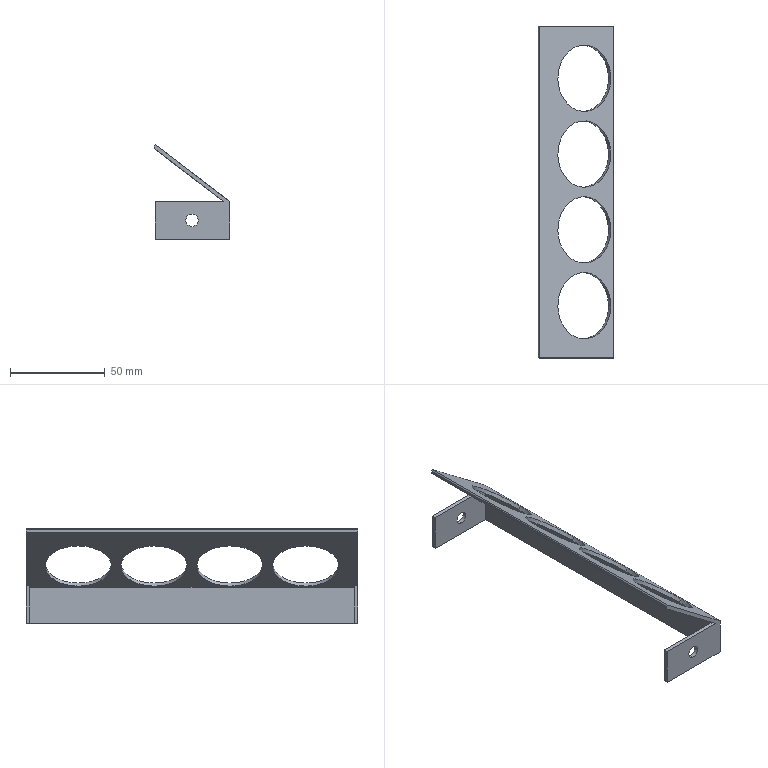Part | SolidWorks | features BaseBody 1 | 1 solid | 27 faces | box 40 x 175 x 50 mm | volume 19089 mm3 | plane 15 | cylinder 12 | commonest cylinder face diameters 35 x8 6.5 x4
STEP:
#1=CARTESIAN_POINT('',(163.696,-4210.973,1848.314));
#2=VERTEX_POINT('',#1);
#3=CARTESIAN_POINT('',(191.569,-4210.973,1827.145));
#4=VERTEX_POINT('',#3);
#5=CARTESIAN_POINT('',(163.696,-4210.973,1848.314));
#6=CARTESIAN_POINT('',(163.696,-4245.973,1848.314));
#7=CARTESIAN_POINT('',(191.569,-4245.973,1827.145));
#8=CARTESIAN_POINT('',(191.569,-4210.973,1827.145));
#9=(BOUNDED_CURVE()B_SPLINE_CURVE(3,(#5,#6,#7,#8),.UNSPECIFIED.,.F.,.F.)B_SPLINE_CURVE_WITH_KNOTS((4,4),(0.,3.142),.UNSPECIFIED.)CURVE()GEOMETRIC_REPRESENTATION_ITEM()RATIONAL_B_SPLINE_CURVE((1.,0.3333,0.3333,1.))REPRESENTATION_ITEM(''));
#10=EDGE_CURVE('',#2,#4,#9,.T.);
#11=ORIENTED_EDGE('',*,*,#10,.F.);
#12=CARTESIAN_POINT('',(164.9,-4210.973,1849.911));
#13=VERTEX_POINT('',#12);
#14=CARTESIAN_POINT('',(167.638,-4210.973,1853.544));
#15=DIRECTION('',(0.6018,0.,0.7986));
#16=VECTOR('',#15,1000.);
#17=LINE('',#14,#16);
#18=EDGE_CURVE('',#2,#13,#17,.T.);
#19=ORIENTED_EDGE('',*,*,#18,.T.);
#20=CARTESIAN_POINT('',(192.773,-4210.973,1828.742));
#21=VERTEX_POINT('',#20);
#22=CARTESIAN_POINT('',(192.773,-4210.973,1828.742));
#23=CARTESIAN_POINT('',(192.773,-4245.973,1828.742));
#24=CARTESIAN_POINT('',(164.9,-4245.973,1849.911));
#25=CARTESIAN_POINT('',(164.9,-4210.973,1849.911));
#26=(BOUNDED_CURVE()B_SPLINE_CURVE(3,(#22,#23,#24,#25),.UNSPECIFIED.,.F.,.T.)B_SPLINE_CURVE_WITH_KNOTS((4,4),(3.142,6.283),.UNSPECIFIED.)CURVE()GEOMETRIC_REPRESENTATION_ITEM()RATIONAL_B_SPLINE_CURVE((1.,0.3333,0.3333,1.))REPRESENTATION_ITEM(''));
#27=EDGE_CURVE('',#21,#13,#26,.T.);
#28=ORIENTED_EDGE('',*,*,#27,.F.);
#29=CARTESIAN_POINT('',(195.59,-4210.973,1832.481));
#30=DIRECTION('',(0.6018,0.,0.7986));
#31=VECTOR('',#30,1000.);
#32=LINE('',#29,#31);
#33=EDGE_CURVE('',#4,#21,#32,.T.);
#34=ORIENTED_EDGE('',*,*,#33,.F.);
#35=EDGE_LOOP('',(#11,#19,#28,#34));
#36=FACE_OUTER_BOUND('',#35,.T.);
#37=CARTESIAN_POINT('',(181.614,-4210.973,1843.013));
#38=DIRECTION('',(0.6018,0.,0.7986));
#39=DIRECTION('',(0.7986,0.,-0.6018));
#40=AXIS2_PLACEMENT_3D('',#37,#38,#39);
#41=CYLINDRICAL_SURFACE('',#40,17.5);
#42=ADVANCED_FACE('',(#36),#41,.F.);
#43=CARTESIAN_POINT('',(192.773,-4250.973,1828.742));
#44=VERTEX_POINT('',#43);
#45=CARTESIAN_POINT('',(164.9,-4250.973,1849.911));
#46=VERTEX_POINT('',#45);
#47=CARTESIAN_POINT('',(192.773,-4250.973,1828.742));
#48=CARTESIAN_POINT('',(192.773,-4285.973,1828.742));
#49=CARTESIAN_POINT('',(164.9,-4285.973,1849.911));
#50=CARTESIAN_POINT('',(164.9,-4250.973,1849.911));
#51=(BOUNDED_CURVE()B_SPLINE_CURVE(3,(#47,#48,#49,#50),.UNSPECIFIED.,.F.,.T.)B_SPLINE_CURVE_WITH_KNOTS((4,4),(0.,3.142),.UNSPECIFIED.)CURVE()GEOMETRIC_REPRESENTATION_ITEM()RATIONAL_B_SPLINE_CURVE((1.,0.3333,0.3333,1.))REPRESENTATION_ITEM(''));
#52=EDGE_CURVE('',#44,#46,#51,.T.);
#53=ORIENTED_EDGE('',*,*,#52,.F.);
#54=CARTESIAN_POINT('',(191.569,-4250.973,1827.145));
#55=VERTEX_POINT('',#54);
#56=CARTESIAN_POINT('',(195.59,-4250.973,1832.481));
#57=DIRECTION('',(-0.6018,0.,-0.7986));
#58=VECTOR('',#57,1000.);
#59=LINE('',#56,#58);
#60=EDGE_CURVE('',#44,#55,#59,.T.);
#61=ORIENTED_EDGE('',*,*,#60,.T.);
#62=CARTESIAN_POINT('',(163.696,-4250.973,1848.314));
#63=VERTEX_POINT('',#62);
#64=CARTESIAN_POINT('',(163.696,-4250.973,1848.314));
#65=CARTESIAN_POINT('',(163.696,-4285.973,1848.314));
#66=CARTESIAN_POINT('',(191.569,-4285.973,1827.145));
#67=CARTESIAN_POINT('',(191.569,-4250.973,1827.145));
#68=(BOUNDED_CURVE()B_SPLINE_CURVE(3,(#64,#65,#66,#67),.UNSPECIFIED.,.F.,.F.)B_SPLINE_CURVE_WITH_KNOTS((4,4),(3.142,6.283),.UNSPECIFIED.)CURVE()GEOMETRIC_REPRESENTATION_ITEM()RATIONAL_B_SPLINE_CURVE((1.,0.3333,0.3333,1.))REPRESENTATION_ITEM(''));
#69=EDGE_CURVE('',#63,#55,#68,.T.);
#70=ORIENTED_EDGE('',*,*,#69,.F.);
#71=CARTESIAN_POINT('',(167.638,-4250.973,1853.544));
#72=DIRECTION('',(-0.6018,0.,-0.7986));
#73=VECTOR('',#72,1000.);
#74=LINE('',#71,#73);
#75=EDGE_CURVE('',#46,#63,#74,.T.);
#76=ORIENTED_EDGE('',*,*,#75,.F.);
#77=EDGE_LOOP('',(#53,#61,#70,#76));
#78=FACE_OUTER_BOUND('',#77,.T.);
#79=CARTESIAN_POINT('',(181.614,-4250.973,1843.013));
#80=DIRECTION('',(-0.6018,0.,-0.7986));
#81=DIRECTION('',(-0.7986,0.,0.6018));
#82=AXIS2_PLACEMENT_3D('',#79,#80,#81);
#83=CYLINDRICAL_SURFACE('',#82,17.5);
#84=ADVANCED_FACE('',(#78),#83,.F.);
#85=CARTESIAN_POINT('',(192.773,-4290.973,1828.742));
#86=VERTEX_POINT('',#85);
#87=CARTESIAN_POINT('',(164.9,-4290.973,1849.911));
#88=VERTEX_POINT('',#87);
#89=CARTESIAN_POINT('',(192.773,-4290.973,1828.742));
#90=CARTESIAN_POINT('',(192.773,-4325.973,1828.742));
#91=CARTESIAN_POINT('',(164.9,-4325.973,1849.911));
#92=CARTESIAN_POINT('',(164.9,-4290.973,1849.911));
#93=(BOUNDED_CURVE()B_SPLINE_CURVE(3,(#89,#90,#91,#92),.UNSPECIFIED.,.F.,.T.)B_SPLINE_CURVE_WITH_KNOTS((4,4),(0.,3.142),.UNSPECIFIED.)CURVE()GEOMETRIC_REPRESENTATION_ITEM()RATIONAL_B_SPLINE_CURVE((1.,0.3333,0.3333,1.))REPRESENTATION_ITEM(''));
#94=EDGE_CURVE('',#86,#88,#93,.T.);
#95=ORIENTED_EDGE('',*,*,#94,.F.);
#96=CARTESIAN_POINT('',(191.569,-4290.973,1827.145));
#97=VERTEX_POINT('',#96);
#98=CARTESIAN_POINT('',(195.59,-4290.973,1832.481));
#99=DIRECTION('',(-0.6018,0.,-0.7986));
#100=VECTOR('',#99,1000.);
#101=LINE('',#98,#100);
#102=EDGE_CURVE('',#86,#97,#101,.T.);
#103=ORIENTED_EDGE('',*,*,#102,.T.);
#104=CARTESIAN_POINT('',(163.696,-4290.973,1848.314));
#105=VERTEX_POINT('',#104);
#106=CARTESIAN_POINT('',(163.696,-4290.973,1848.314));
#107=CARTESIAN_POINT('',(163.696,-4325.973,1848.314));
#108=CARTESIAN_POINT('',(191.569,-4325.973,1827.145));
#109=CARTESIAN_POINT('',(191.569,-4290.973,1827.145));
#110=(BOUNDED_CURVE()B_SPLINE_CURVE(3,(#106,#107,#108,#109),.UNSPECIFIED.,.F.,.F.)B_SPLINE_CURVE_WITH_KNOTS((4,4),(3.142,6.283),.UNSPECIFIED.)CURVE()GEOMETRIC_REPRESENTATION_ITEM()RATIONAL_B_SPLINE_CURVE((1.,0.3333,0.3333,1.))REPRESENTATION_ITEM(''));
#111=EDGE_CURVE('',#105,#97,#110,.T.);
#112=ORIENTED_EDGE('',*,*,#111,.F.);
#113=CARTESIAN_POINT('',(167.638,-4290.973,1853.544));
#114=DIRECTION('',(-0.6018,0.,-0.7986));
#115=VECTOR('',#114,1000.);
#116=LINE('',#113,#115);
#117=EDGE_CURVE('',#88,#105,#116,.T.);
#118=ORIENTED_EDGE('',*,*,#117,.F.);
#119=EDGE_LOOP('',(#95,#103,#112,#118));
#120=FACE_OUTER_BOUND('',#119,.T.);
#121=CARTESIAN_POINT('',(181.614,-4290.973,1843.013));
#122=DIRECTION('',(-0.6018,0.,-0.7986));
#123=DIRECTION('',(-0.7986,0.,0.6018));
#124=AXIS2_PLACEMENT_3D('',#121,#122,#123);
#125=CYLINDRICAL_SURFACE('',#124,17.5);
#126=ADVANCED_FACE('',(#120),#125,.F.);
#127=CARTESIAN_POINT('',(163.696,-4170.973,1848.314));
#128=VERTEX_POINT('',#127);
#129=CARTESIAN_POINT('',(191.569,-4170.973,1827.145));
#130=VERTEX_POINT('',#129);
#131=CARTESIAN_POINT('',(163.696,-4170.973,1848.314));
#132=CARTESIAN_POINT('',(163.696,-4205.973,1848.314));
#133=CARTESIAN_POINT('',(191.569,-4205.973,1827.145));
#134=CARTESIAN_POINT('',(191.569,-4170.973,1827.145));
#135=(BOUNDED_CURVE()B_SPLINE_CURVE(3,(#131,#132,#133,#134),.UNSPECIFIED.,.F.,.T.)B_SPLINE_CURVE_WITH_KNOTS((4,4),(0.,3.142),.UNSPECIFIED.)CURVE()GEOMETRIC_REPRESENTATION_ITEM()RATIONAL_B_SPLINE_CURVE((1.,0.3333,0.3333,1.))REPRESENTATION_ITEM(''));
#136=EDGE_CURVE('',#128,#130,#135,.T.);
#137=ORIENTED_EDGE('',*,*,#136,.F.);
#138=CARTESIAN_POINT('',(164.9,-4170.973,1849.911));
#139=VERTEX_POINT('',#138);
#140=CARTESIAN_POINT('',(167.638,-4170.973,1853.544));
#141=DIRECTION('',(0.6018,0.,0.7986));
#142=VECTOR('',#141,1000.);
#143=LINE('',#140,#142);
#144=EDGE_CURVE('',#128,#139,#143,.T.);
#145=ORIENTED_EDGE('',*,*,#144,.T.);
#146=CARTESIAN_POINT('',(192.773,-4170.973,1828.742));
#147=VERTEX_POINT('',#146);
#148=CARTESIAN_POINT('',(192.773,-4170.973,1828.742));
#149=CARTESIAN_POINT('',(192.773,-4205.973,1828.742));
#150=CARTESIAN_POINT('',(164.9,-4205.973,1849.911));
#151=CARTESIAN_POINT('',(164.9,-4170.973,1849.911));
#152=(BOUNDED_CURVE()B_SPLINE_CURVE(3,(#148,#149,#150,#151),.UNSPECIFIED.,.F.,.T.)B_SPLINE_CURVE_WITH_KNOTS((4,4),(3.142,6.283),.UNSPECIFIED.)CURVE()GEOMETRIC_REPRESENTATION_ITEM()RATIONAL_B_SPLINE_CURVE((1.,0.3333,0.3333,1.))REPRESENTATION_ITEM(''));
#153=EDGE_CURVE('',#147,#139,#152,.T.);
#154=ORIENTED_EDGE('',*,*,#153,.F.);
#155=CARTESIAN_POINT('',(195.59,-4170.973,1832.481));
#156=DIRECTION('',(0.6018,0.,0.7986));
#157=VECTOR('',#156,1000.);
#158=LINE('',#155,#157);
#159=EDGE_CURVE('',#130,#147,#158,.T.);
#160=ORIENTED_EDGE('',*,*,#159,.F.);
#161=EDGE_LOOP('',(#137,#145,#154,#160));
#162=FACE_OUTER_BOUND('',#161,.T.);
#163=CARTESIAN_POINT('',(181.614,-4170.973,1843.013));
#164=DIRECTION('',(0.6018,0.,0.7986));
#165=DIRECTION('',(0.7986,0.,-0.6018));
#166=AXIS2_PLACEMENT_3D('',#163,#164,#165);
#167=CYLINDRICAL_SURFACE('',#166,17.5);
#168=ADVANCED_FACE('',(#162),#167,.F.);
#169=CARTESIAN_POINT('',(174.446,-4143.473,1820.721));
#170=VERTEX_POINT('',#169);
#171=CARTESIAN_POINT('',(174.446,-4143.473,1814.221));
#172=VERTEX_POINT('',#171);
#173=CARTESIAN_POINT('',(174.446,-4143.473,1817.471));
#174=DIRECTION('',(0.,-1.,0.));
#175=DIRECTION('',(0.,0.,-1.));
#176=AXIS2_PLACEMENT_3D('',#173,#174,#175);
#177=CIRCLE('',#176,3.25);
#178=EDGE_CURVE('',#170,#172,#177,.T.);
#179=ORIENTED_EDGE('',*,*,#178,.F.);
#180=CARTESIAN_POINT('',(174.446,-4145.473,1820.721));
#181=VERTEX_POINT('',#180);
#182=CARTESIAN_POINT('',(174.446,-4339.435,1820.721));
#183=DIRECTION('',(0.,-1.,0.));
#184=VECTOR('',#183,1000.);
#185=LINE('',#182,#184);
#186=EDGE_CURVE('',#170,#181,#185,.T.);
#187=ORIENTED_EDGE('',*,*,#186,.T.);
#188=CARTESIAN_POINT('',(174.446,-4145.473,1814.221));
#189=VERTEX_POINT('',#188);
#190=CARTESIAN_POINT('',(174.446,-4145.473,1817.471));
#191=DIRECTION('',(0.,1.,0.));
#192=DIRECTION('',(0.,0.,-1.));
#193=AXIS2_PLACEMENT_3D('',#190,#191,#192);
#194=CIRCLE('',#193,3.25);
#195=EDGE_CURVE('',#189,#181,#194,.T.);
#196=ORIENTED_EDGE('',*,*,#195,.F.);
#197=CARTESIAN_POINT('',(174.446,-4339.435,1814.221));
#198=DIRECTION('',(0.,-1.,0.));
#199=VECTOR('',#198,1000.);
#200=LINE('',#197,#199);
#201=EDGE_CURVE('',#172,#189,#200,.T.);
#202=ORIENTED_EDGE('',*,*,#201,.F.);
#203=EDGE_LOOP('',(#179,#187,#196,#202));
#204=FACE_OUTER_BOUND('',#203,.T.);
#205=CARTESIAN_POINT('',(174.446,-4339.435,1817.471));
#206=DIRECTION('',(0.,-1.,0.));
#207=DIRECTION('',(0.,0.,-1.));
#208=AXIS2_PLACEMENT_3D('',#205,#206,#207);
#209=CYLINDRICAL_SURFACE('',#208,3.25);
#210=ADVANCED_FACE('',(#204),#209,.F.);
#211=CARTESIAN_POINT('',(174.446,-4316.473,1820.721));
#212=VERTEX_POINT('',#211);
#213=CARTESIAN_POINT('',(174.446,-4316.473,1814.221));
#214=VERTEX_POINT('',#213);
#215=CARTESIAN_POINT('',(174.446,-4316.473,1817.471));
#216=DIRECTION('',(0.,-1.,0.));
#217=DIRECTION('',(0.,0.,-1.));
#218=AXIS2_PLACEMENT_3D('',#215,#216,#217);
#219=CIRCLE('',#218,3.25);
#220=EDGE_CURVE('',#212,#214,#219,.T.);
#221=ORIENTED_EDGE('',*,*,#220,.F.);
#222=CARTESIAN_POINT('',(174.446,-4318.473,1820.721));
#223=VERTEX_POINT('',#222);
#224=CARTESIAN_POINT('',(174.446,-4339.435,1820.721));
#225=DIRECTION('',(0.,-1.,0.));
#226=VECTOR('',#225,1000.);
#227=LINE('',#224,#226);
#228=EDGE_CURVE('',#212,#223,#227,.T.);
#229=ORIENTED_EDGE('',*,*,#228,.T.);
#230=CARTESIAN_POINT('',(174.446,-4318.473,1814.221));
#231=VERTEX_POINT('',#230);
#232=CARTESIAN_POINT('',(174.446,-4318.473,1817.471));
#233=DIRECTION('',(0.,1.,0.));
#234=DIRECTION('',(0.,0.,-1.));
#235=AXIS2_PLACEMENT_3D('',#232,#233,#234);
#236=CIRCLE('',#235,3.25);
#237=EDGE_CURVE('',#231,#223,#236,.T.);
#238=ORIENTED_EDGE('',*,*,#237,.F.);
#239=CARTESIAN_POINT('',(174.446,-4339.435,1814.221));
#240=DIRECTION('',(0.,-1.,0.));
#241=VECTOR('',#240,1000.);
#242=LINE('',#239,#241);
#243=EDGE_CURVE('',#214,#231,#242,.T.);
#244=ORIENTED_EDGE('',*,*,#243,.F.);
#245=EDGE_LOOP('',(#221,#229,#238,#244));
#246=FACE_OUTER_BOUND('',#245,.T.);
#247=CARTESIAN_POINT('',(174.446,-4339.435,1817.471));
#248=DIRECTION('',(0.,-1.,0.));
#249=DIRECTION('',(0.,0.,-1.));
#250=AXIS2_PLACEMENT_3D('',#247,#248,#249);
#251=CYLINDRICAL_SURFACE('',#250,3.25);
#252=ADVANCED_FACE('',(#246),#251,.F.);
#253=CARTESIAN_POINT('',(194.446,-4143.473,1827.471));
#254=VERTEX_POINT('',#253);
#255=CARTESIAN_POINT('',(154.946,-4143.473,1857.471));
#256=VERTEX_POINT('',#255);
#257=CARTESIAN_POINT('',(154.946,-4143.473,1857.471));
#258=DIRECTION('',(-0.7964,0.,0.6048));
#259=VECTOR('',#258,1000.);
#260=LINE('',#257,#259);
#261=EDGE_CURVE('',#254,#256,#260,.T.);
#262=ORIENTED_EDGE('',*,*,#261,.T.);
#263=CARTESIAN_POINT('',(154.946,-4318.473,1857.471));
#264=VERTEX_POINT('',#263);
#265=CARTESIAN_POINT('',(154.946,-4143.473,1857.471));
#266=DIRECTION('',(0.,-1.,0.));
#267=VECTOR('',#266,1000.);
#268=LINE('',#265,#267);
#269=EDGE_CURVE('',#256,#264,#268,.T.);
#270=ORIENTED_EDGE('',*,*,#269,.T.);
#271=CARTESIAN_POINT('',(194.446,-4318.473,1827.471));
#272=VERTEX_POINT('',#271);
#273=CARTESIAN_POINT('',(154.946,-4318.473,1857.471));
#274=DIRECTION('',(0.7964,0.,-0.6048));
#275=VECTOR('',#274,1000.);
#276=LINE('',#273,#275);
#277=EDGE_CURVE('',#264,#272,#276,.T.);
#278=ORIENTED_EDGE('',*,*,#277,.T.);
#279=CARTESIAN_POINT('',(194.446,-4143.473,1827.471));
#280=DIRECTION('',(0.,1.,0.));
#281=VECTOR('',#280,1000.);
#282=LINE('',#279,#281);
#283=EDGE_CURVE('',#272,#254,#282,.T.);
#284=ORIENTED_EDGE('',*,*,#283,.T.);
#285=EDGE_LOOP('',(#262,#270,#278,#284));
#286=FACE_OUTER_BOUND('',#285,.T.);
#287=ORIENTED_EDGE('',*,*,#27,.T.);
#288=CARTESIAN_POINT('',(164.9,-4210.973,1849.911));
#289=CARTESIAN_POINT('',(164.9,-4175.973,1849.911));
#290=CARTESIAN_POINT('',(192.773,-4175.973,1828.742));
#291=CARTESIAN_POINT('',(192.773,-4210.973,1828.742));
#292=(BOUNDED_CURVE()B_SPLINE_CURVE(3,(#288,#289,#290,#291),.UNSPECIFIED.,.F.,.F.)B_SPLINE_CURVE_WITH_KNOTS((4,4),(0.,3.142),.UNSPECIFIED.)CURVE()GEOMETRIC_REPRESENTATION_ITEM()RATIONAL_B_SPLINE_CURVE((1.,0.3333,0.3333,1.))REPRESENTATION_ITEM(''));
#293=EDGE_CURVE('',#13,#21,#292,.T.);
#294=ORIENTED_EDGE('',*,*,#293,.T.);
#295=EDGE_LOOP('',(#287,#294));
#296=FACE_BOUND('',#295,.T.);
#297=CARTESIAN_POINT('',(164.9,-4250.973,1849.911));
#298=CARTESIAN_POINT('',(164.9,-4215.973,1849.911));
#299=CARTESIAN_POINT('',(192.773,-4215.973,1828.742));
#300=CARTESIAN_POINT('',(192.773,-4250.973,1828.742));
#301=(BOUNDED_CURVE()B_SPLINE_CURVE(3,(#297,#298,#299,#300),.UNSPECIFIED.,.F.,.F.)B_SPLINE_CURVE_WITH_KNOTS((4,4),(3.142,6.283),.UNSPECIFIED.)CURVE()GEOMETRIC_REPRESENTATION_ITEM()RATIONAL_B_SPLINE_CURVE((1.,0.3333,0.3333,1.))REPRESENTATION_ITEM(''));
#302=EDGE_CURVE('',#46,#44,#301,.T.);
#303=ORIENTED_EDGE('',*,*,#302,.T.);
#304=ORIENTED_EDGE('',*,*,#52,.T.);
#305=EDGE_LOOP('',(#303,#304));
#306=FACE_BOUND('',#305,.T.);
#307=CARTESIAN_POINT('',(164.9,-4290.973,1849.911));
#308=CARTESIAN_POINT('',(164.9,-4255.973,1849.911));
#309=CARTESIAN_POINT('',(192.773,-4255.973,1828.742));
#310=CARTESIAN_POINT('',(192.773,-4290.973,1828.742));
#311=(BOUNDED_CURVE()B_SPLINE_CURVE(3,(#307,#308,#309,#310),.UNSPECIFIED.,.F.,.F.)B_SPLINE_CURVE_WITH_KNOTS((4,4),(3.142,6.283),.UNSPECIFIED.)CURVE()GEOMETRIC_REPRESENTATION_ITEM()RATIONAL_B_SPLINE_CURVE((1.,0.3333,0.3333,1.))REPRESENTATION_ITEM(''));
#312=EDGE_CURVE('',#88,#86,#311,.T.);
#313=ORIENTED_EDGE('',*,*,#312,.T.);
#314=ORIENTED_EDGE('',*,*,#94,.T.);
#315=EDGE_LOOP('',(#313,#314));
#316=FACE_BOUND('',#315,.T.);
#317=ORIENTED_EDGE('',*,*,#153,.T.);
#318=CARTESIAN_POINT('',(164.9,-4170.973,1849.911));
#319=CARTESIAN_POINT('',(164.9,-4135.973,1849.911));
#320=CARTESIAN_POINT('',(192.773,-4135.973,1828.742));
#321=CARTESIAN_POINT('',(192.773,-4170.973,1828.742));
#322=(BOUNDED_CURVE()B_SPLINE_CURVE(3,(#318,#319,#320,#321),.UNSPECIFIED.,.F.,.F.)B_SPLINE_CURVE_WITH_KNOTS((4,4),(0.,3.142),.UNSPECIFIED.)CURVE()GEOMETRIC_REPRESENTATION_ITEM()RATIONAL_B_SPLINE_CURVE((1.,0.3333,0.3333,1.))REPRESENTATION_ITEM(''));
#323=EDGE_CURVE('',#139,#147,#322,.T.);
#324=ORIENTED_EDGE('',*,*,#323,.T.);
#325=EDGE_LOOP('',(#317,#324));
#326=FACE_BOUND('',#325,.T.);
#327=CARTESIAN_POINT('',(154.946,-4143.473,1857.471));
#328=DIRECTION('',(0.6048,0.,0.7964));
#329=DIRECTION('',(0.7964,0.,-0.6048));
#330=AXIS2_PLACEMENT_3D('',#327,#328,#329);
#331=PLANE('',#330);
#332=ADVANCED_FACE('',(#286,#296,#306,#316,#326),#331,.T.);
#333=ORIENTED_EDGE('',*,*,#269,.F.);
#334=CARTESIAN_POINT('',(154.446,-4143.473,1856.813));
#335=VERTEX_POINT('',#334);
#336=CARTESIAN_POINT('',(153.736,-4143.473,1855.879));
#337=DIRECTION('',(-0.6048,0.,-0.7964));
#338=VECTOR('',#337,1000.);
#339=LINE('',#336,#338);
#340=EDGE_CURVE('',#256,#335,#339,.T.);
#341=ORIENTED_EDGE('',*,*,#340,.T.);
#342=CARTESIAN_POINT('',(154.446,-4318.473,1856.813));
#343=VERTEX_POINT('',#342);
#344=CARTESIAN_POINT('',(154.446,-4143.473,1856.813));
#345=DIRECTION('',(0.,-1.,0.));
#346=VECTOR('',#345,1000.);
#347=LINE('',#344,#346);
#348=EDGE_CURVE('',#335,#343,#347,.T.);
#349=ORIENTED_EDGE('',*,*,#348,.T.);
#350=CARTESIAN_POINT('',(153.736,-4318.473,1855.879));
#351=DIRECTION('',(0.6048,0.,0.7964));
#352=VECTOR('',#351,1000.);
#353=LINE('',#350,#352);
#354=EDGE_CURVE('',#343,#264,#353,.T.);
#355=ORIENTED_EDGE('',*,*,#354,.T.);
#356=EDGE_LOOP('',(#333,#341,#349,#355));
#357=FACE_OUTER_BOUND('',#356,.T.);
#358=CARTESIAN_POINT('',(153.736,-4143.473,1855.879));
#359=DIRECTION('',(-0.7964,0.,0.6048));
#360=DIRECTION('',(0.6048,0.,0.7964));
#361=AXIS2_PLACEMENT_3D('',#358,#359,#360);
#362=PLANE('',#361);
#363=ADVANCED_FACE('',(#357),#362,.T.);
#364=CARTESIAN_POINT('',(174.446,-4143.473,1817.471));
#365=DIRECTION('',(0.,-1.,0.));
#366=DIRECTION('',(0.,0.,-1.));
#367=AXIS2_PLACEMENT_3D('',#364,#365,#366);
#368=CIRCLE('',#367,3.25);
#369=EDGE_CURVE('',#172,#170,#368,.T.);
#370=ORIENTED_EDGE('',*,*,#369,.T.);
#371=ORIENTED_EDGE('',*,*,#178,.T.);
#372=EDGE_LOOP('',(#370,#371));
#373=FACE_BOUND('',#372,.T.);
#374=CARTESIAN_POINT('',(154.946,-4143.473,1827.471));
#375=VERTEX_POINT('',#374);
#376=CARTESIAN_POINT('',(191.139,-4143.473,1827.471));
#377=VERTEX_POINT('',#376);
#378=CARTESIAN_POINT('',(174.696,-4143.473,1827.471));
#379=DIRECTION('',(1.,0.,0.));
#380=VECTOR('',#379,1000.);
#381=LINE('',#378,#380);
#382=EDGE_CURVE('',#375,#377,#381,.T.);
#383=ORIENTED_EDGE('',*,*,#382,.T.);
#384=CARTESIAN_POINT('',(154.446,-4143.473,1855.34));
#385=VERTEX_POINT('',#384);
#386=CARTESIAN_POINT('',(191.139,-4143.473,1827.471));
#387=DIRECTION('',(-0.7964,0.,0.6048));
#388=VECTOR('',#387,1000.);
#389=LINE('',#386,#388);
#390=EDGE_CURVE('',#377,#385,#389,.T.);
#391=ORIENTED_EDGE('',*,*,#390,.T.);
#392=CARTESIAN_POINT('',(154.446,-4143.473,1817.471));
#393=DIRECTION('',(0.,0.,1.));
#394=VECTOR('',#393,1000.);
#395=LINE('',#392,#394);
#396=EDGE_CURVE('',#385,#335,#395,.T.);
#397=ORIENTED_EDGE('',*,*,#396,.T.);
#398=ORIENTED_EDGE('',*,*,#340,.F.);
#399=ORIENTED_EDGE('',*,*,#261,.F.);
#400=CARTESIAN_POINT('',(194.446,-4143.473,1807.471));
#401=VERTEX_POINT('',#400);
#402=CARTESIAN_POINT('',(194.446,-4143.473,1817.471));
#403=DIRECTION('',(0.,0.,-1.));
#404=VECTOR('',#403,1000.);
#405=LINE('',#402,#404);
#406=EDGE_CURVE('',#254,#401,#405,.T.);
#407=ORIENTED_EDGE('',*,*,#406,.T.);
#408=CARTESIAN_POINT('',(154.946,-4143.473,1807.471));
#409=VERTEX_POINT('',#408);
#410=CARTESIAN_POINT('',(174.696,-4143.473,1807.471));
#411=DIRECTION('',(-1.,0.,0.));
#412=VECTOR('',#411,1000.);
#413=LINE('',#410,#412);
#414=EDGE_CURVE('',#401,#409,#413,.T.);
#415=ORIENTED_EDGE('',*,*,#414,.T.);
#416=CARTESIAN_POINT('',(154.946,-4143.473,1817.471));
#417=DIRECTION('',(0.,0.,1.));
#418=VECTOR('',#417,1000.);
#419=LINE('',#416,#418);
#420=EDGE_CURVE('',#409,#375,#419,.T.);
#421=ORIENTED_EDGE('',*,*,#420,.T.);
#422=EDGE_LOOP('',(#383,#391,#397,#398,#399,#407,#415,#421));
#423=FACE_OUTER_BOUND('',#422,.T.);
#424=CARTESIAN_POINT('',(174.696,-4143.473,1817.471));
#425=DIRECTION('',(0.,1.,0.));
#426=DIRECTION('',(0.,0.,1.));
#427=AXIS2_PLACEMENT_3D('',#424,#425,#426);
#428=PLANE('',#427);
#429=ADVANCED_FACE('',(#373,#423),#428,.T.);
#430=CARTESIAN_POINT('',(194.446,-4318.473,1807.471));
#431=VERTEX_POINT('',#430);
#432=CARTESIAN_POINT('',(194.446,-4318.473,1807.471));
#433=DIRECTION('',(0.,1.,0.));
#434=VECTOR('',#433,1000.);
#435=LINE('',#432,#434);
#436=EDGE_CURVE('',#431,#401,#435,.T.);
#437=ORIENTED_EDGE('',*,*,#436,.T.);
#438=ORIENTED_EDGE('',*,*,#406,.F.);
#439=ORIENTED_EDGE('',*,*,#283,.F.);
#440=CARTESIAN_POINT('',(194.446,-4318.473,1827.471));
#441=DIRECTION('',(0.,0.,-1.));
#442=VECTOR('',#441,1000.);
#443=LINE('',#440,#442);
#444=EDGE_CURVE('',#272,#431,#443,.T.);
#445=ORIENTED_EDGE('',*,*,#444,.T.);
#446=EDGE_LOOP('',(#437,#438,#439,#445));
#447=FACE_OUTER_BOUND('',#446,.T.);
#448=CARTESIAN_POINT('',(194.446,-4318.473,1827.471));
#449=DIRECTION('',(1.,0.,0.));
#450=DIRECTION('',(0.,0.,-1.));
#451=AXIS2_PLACEMENT_3D('',#448,#449,#450);
#452=PLANE('',#451);
#453=ADVANCED_FACE('',(#447),#452,.T.);
#454=ORIENTED_EDGE('',*,*,#237,.T.);
#455=CARTESIAN_POINT('',(174.446,-4318.473,1817.471));
#456=DIRECTION('',(0.,1.,0.));
#457=DIRECTION('',(0.,0.,-1.));
#458=AXIS2_PLACEMENT_3D('',#455,#456,#457);
#459=CIRCLE('',#458,3.25);
#460=EDGE_CURVE('',#223,#231,#459,.T.);
#461=ORIENTED_EDGE('',*,*,#460,.T.);
#462=EDGE_LOOP('',(#454,#461));
#463=FACE_BOUND('',#462,.T.);
#464=ORIENTED_EDGE('',*,*,#277,.F.);
#465=ORIENTED_EDGE('',*,*,#354,.F.);
#466=CARTESIAN_POINT('',(154.446,-4318.473,1855.34));
#467=VERTEX_POINT('',#466);
#468=CARTESIAN_POINT('',(154.446,-4318.473,1817.471));
#469=DIRECTION('',(0.,0.,-1.));
#470=VECTOR('',#469,1000.);
#471=LINE('',#468,#470);
#472=EDGE_CURVE('',#343,#467,#471,.T.);
#473=ORIENTED_EDGE('',*,*,#472,.T.);
#474=CARTESIAN_POINT('',(191.139,-4318.473,1827.471));
#475=VERTEX_POINT('',#474);
#476=CARTESIAN_POINT('',(154.446,-4318.473,1855.34));
#477=DIRECTION('',(0.7964,0.,-0.6048));
#478=VECTOR('',#477,1000.);
#479=LINE('',#476,#478);
#480=EDGE_CURVE('',#467,#475,#479,.T.);
#481=ORIENTED_EDGE('',*,*,#480,.T.);
#482=CARTESIAN_POINT('',(154.946,-4318.473,1827.471));
#483=VERTEX_POINT('',#482);
#484=CARTESIAN_POINT('',(174.696,-4318.473,1827.471));
#485=DIRECTION('',(-1.,0.,0.));
#486=VECTOR('',#485,1000.);
#487=LINE('',#484,#486);
#488=EDGE_CURVE('',#475,#483,#487,.T.);
#489=ORIENTED_EDGE('',*,*,#488,.T.);
#490=CARTESIAN_POINT('',(154.946,-4318.473,1807.471));
#491=VERTEX_POINT('',#490);
#492=CARTESIAN_POINT('',(154.946,-4318.473,1817.471));
#493=DIRECTION('',(0.,0.,-1.));
#494=VECTOR('',#493,1000.);
#495=LINE('',#492,#494);
#496=EDGE_CURVE('',#483,#491,#495,.T.);
#497=ORIENTED_EDGE('',*,*,#496,.T.);
#498=CARTESIAN_POINT('',(174.696,-4318.473,1807.471));
#499=DIRECTION('',(1.,0.,0.));
#500=VECTOR('',#499,1000.);
#501=LINE('',#498,#500);
#502=EDGE_CURVE('',#491,#431,#501,.T.);
#503=ORIENTED_EDGE('',*,*,#502,.T.);
#504=ORIENTED_EDGE('',*,*,#444,.F.);
#505=EDGE_LOOP('',(#464,#465,#473,#481,#489,#497,#503,#504));
#506=FACE_OUTER_BOUND('',#505,.T.);
#507=CARTESIAN_POINT('',(174.696,-4318.473,1817.471));
#508=DIRECTION('',(0.,-1.,0.));
#509=DIRECTION('',(0.,0.,-1.));
#510=AXIS2_PLACEMENT_3D('',#507,#508,#509);
#511=PLANE('',#510);
#512=ADVANCED_FACE('',(#463,#506),#511,.T.);
#513=ORIENTED_EDGE('',*,*,#18,.F.);
#514=CARTESIAN_POINT('',(191.569,-4210.973,1827.145));
#515=CARTESIAN_POINT('',(191.569,-4175.973,1827.145));
#516=CARTESIAN_POINT('',(163.696,-4175.973,1848.314));
#517=CARTESIAN_POINT('',(163.696,-4210.973,1848.314));
#518=(BOUNDED_CURVE()B_SPLINE_CURVE(3,(#514,#515,#516,#517),.UNSPECIFIED.,.F.,.T.)B_SPLINE_CURVE_WITH_KNOTS((4,4),(3.142,6.283),.UNSPECIFIED.)CURVE()GEOMETRIC_REPRESENTATION_ITEM()RATIONAL_B_SPLINE_CURVE((1.,0.3333,0.3333,1.))REPRESENTATION_ITEM(''));
#519=EDGE_CURVE('',#4,#2,#518,.T.);
#520=ORIENTED_EDGE('',*,*,#519,.F.);
#521=ORIENTED_EDGE('',*,*,#33,.T.);
#522=ORIENTED_EDGE('',*,*,#293,.F.);
#523=EDGE_LOOP('',(#513,#520,#521,#522));
#524=FACE_OUTER_BOUND('',#523,.T.);
#525=CARTESIAN_POINT('',(181.614,-4210.973,1843.013));
#526=DIRECTION('',(0.6018,0.,0.7986));
#527=DIRECTION('',(0.7986,0.,-0.6018));
#528=AXIS2_PLACEMENT_3D('',#525,#526,#527);
#529=CYLINDRICAL_SURFACE('',#528,17.5);
#530=ADVANCED_FACE('',(#524),#529,.F.);
#531=ORIENTED_EDGE('',*,*,#60,.F.);
#532=ORIENTED_EDGE('',*,*,#302,.F.);
#533=ORIENTED_EDGE('',*,*,#75,.T.);
#534=CARTESIAN_POINT('',(191.569,-4250.973,1827.145));
#535=CARTESIAN_POINT('',(191.569,-4215.973,1827.145));
#536=CARTESIAN_POINT('',(163.696,-4215.973,1848.314));
#537=CARTESIAN_POINT('',(163.696,-4250.973,1848.314));
#538=(BOUNDED_CURVE()B_SPLINE_CURVE(3,(#534,#535,#536,#537),.UNSPECIFIED.,.F.,.F.)B_SPLINE_CURVE_WITH_KNOTS((4,4),(0.,3.142),.UNSPECIFIED.)CURVE()GEOMETRIC_REPRESENTATION_ITEM()RATIONAL_B_SPLINE_CURVE((1.,0.3333,0.3333,1.))REPRESENTATION_ITEM(''));
#539=EDGE_CURVE('',#55,#63,#538,.T.);
#540=ORIENTED_EDGE('',*,*,#539,.F.);
#541=EDGE_LOOP('',(#531,#532,#533,#540));
#542=FACE_OUTER_BOUND('',#541,.T.);
#543=CARTESIAN_POINT('',(181.614,-4250.973,1843.013));
#544=DIRECTION('',(-0.6018,0.,-0.7986));
#545=DIRECTION('',(-0.7986,0.,0.6018));
#546=AXIS2_PLACEMENT_3D('',#543,#544,#545);
#547=CYLINDRICAL_SURFACE('',#546,17.5);
#548=ADVANCED_FACE('',(#542),#547,.F.);
#549=ORIENTED_EDGE('',*,*,#102,.F.);
#550=ORIENTED_EDGE('',*,*,#312,.F.);
#551=ORIENTED_EDGE('',*,*,#117,.T.);
#552=CARTESIAN_POINT('',(191.569,-4290.973,1827.145));
#553=CARTESIAN_POINT('',(191.569,-4255.973,1827.145));
#554=CARTESIAN_POINT('',(163.696,-4255.973,1848.314));
#555=CARTESIAN_POINT('',(163.696,-4290.973,1848.314));
#556=(BOUNDED_CURVE()B_SPLINE_CURVE(3,(#552,#553,#554,#555),.UNSPECIFIED.,.F.,.F.)B_SPLINE_CURVE_WITH_KNOTS((4,4),(0.,3.142),.UNSPECIFIED.)CURVE()GEOMETRIC_REPRESENTATION_ITEM()RATIONAL_B_SPLINE_CURVE((1.,0.3333,0.3333,1.))REPRESENTATION_ITEM(''));
#557=EDGE_CURVE('',#97,#105,#556,.T.);
#558=ORIENTED_EDGE('',*,*,#557,.F.);
#559=EDGE_LOOP('',(#549,#550,#551,#558));
#560=FACE_OUTER_BOUND('',#559,.T.);
#561=CARTESIAN_POINT('',(181.614,-4290.973,1843.013));
#562=DIRECTION('',(-0.6018,0.,-0.7986));
#563=DIRECTION('',(-0.7986,0.,0.6018));
#564=AXIS2_PLACEMENT_3D('',#561,#562,#563);
#565=CYLINDRICAL_SURFACE('',#564,17.5);
#566=ADVANCED_FACE('',(#560),#565,.F.);
#567=ORIENTED_EDGE('',*,*,#144,.F.);
#568=CARTESIAN_POINT('',(191.569,-4170.973,1827.145));
#569=CARTESIAN_POINT('',(191.569,-4135.973,1827.145));
#570=CARTESIAN_POINT('',(163.696,-4135.973,1848.314));
#571=CARTESIAN_POINT('',(163.696,-4170.973,1848.314));
#572=(BOUNDED_CURVE()B_SPLINE_CURVE(3,(#568,#569,#570,#571),.UNSPECIFIED.,.F.,.F.)B_SPLINE_CURVE_WITH_KNOTS((4,4),(3.142,6.283),.UNSPECIFIED.)CURVE()GEOMETRIC_REPRESENTATION_ITEM()RATIONAL_B_SPLINE_CURVE((1.,0.3333,0.3333,1.))REPRESENTATION_ITEM(''));
#573=EDGE_CURVE('',#130,#128,#572,.T.);
#574=ORIENTED_EDGE('',*,*,#573,.F.);
#575=ORIENTED_EDGE('',*,*,#159,.T.);
#576=ORIENTED_EDGE('',*,*,#323,.F.);
#577=EDGE_LOOP('',(#567,#574,#575,#576));
#578=FACE_OUTER_BOUND('',#577,.T.);
#579=CARTESIAN_POINT('',(181.614,-4170.973,1843.013));
#580=DIRECTION('',(0.6018,0.,0.7986));
#581=DIRECTION('',(0.7986,0.,-0.6018));
#582=AXIS2_PLACEMENT_3D('',#579,#580,#581);
#583=CYLINDRICAL_SURFACE('',#582,17.5);
#584=ADVANCED_FACE('',(#578),#583,.F.);
#585=ORIENTED_EDGE('',*,*,#396,.F.);
#586=CARTESIAN_POINT('',(154.446,-4142.973,1855.34));
#587=DIRECTION('',(0.,1.,0.));
#588=VECTOR('',#587,1000.);
#589=LINE('',#586,#588);
#590=EDGE_CURVE('',#467,#385,#589,.T.);
#591=ORIENTED_EDGE('',*,*,#590,.F.);
#592=ORIENTED_EDGE('',*,*,#472,.F.);
#593=ORIENTED_EDGE('',*,*,#348,.F.);
#594=EDGE_LOOP('',(#585,#591,#592,#593));
#595=FACE_OUTER_BOUND('',#594,.T.);
#596=CARTESIAN_POINT('',(154.446,-4142.973,172.471));
#597=DIRECTION('',(1.,0.,0.));
#598=DIRECTION('',(0.,0.,-1.));
#599=AXIS2_PLACEMENT_3D('',#596,#597,#598);
#600=PLANE('',#599);
#601=ADVANCED_FACE('',(#595),#600,.F.);
#602=ORIENTED_EDGE('',*,*,#186,.F.);
#603=ORIENTED_EDGE('',*,*,#369,.F.);
#604=ORIENTED_EDGE('',*,*,#201,.T.);
#605=CARTESIAN_POINT('',(174.446,-4145.473,1817.471));
#606=DIRECTION('',(0.,1.,0.));
#607=DIRECTION('',(0.,0.,-1.));
#608=AXIS2_PLACEMENT_3D('',#605,#606,#607);
#609=CIRCLE('',#608,3.25);
#610=EDGE_CURVE('',#181,#189,#609,.T.);
#611=ORIENTED_EDGE('',*,*,#610,.F.);
#612=EDGE_LOOP('',(#602,#603,#604,#611));
#613=FACE_OUTER_BOUND('',#612,.T.);
#614=CARTESIAN_POINT('',(174.446,-4339.435,1817.471));
#615=DIRECTION('',(0.,-1.,0.));
#616=DIRECTION('',(0.,0.,-1.));
#617=AXIS2_PLACEMENT_3D('',#614,#615,#616);
#618=CYLINDRICAL_SURFACE('',#617,3.25);
#619=ADVANCED_FACE('',(#613),#618,.F.);
#620=ORIENTED_EDGE('',*,*,#573,.T.);
#621=ORIENTED_EDGE('',*,*,#136,.T.);
#622=EDGE_LOOP('',(#620,#621));
#623=FACE_BOUND('',#622,.T.);
#624=ORIENTED_EDGE('',*,*,#111,.T.);
#625=ORIENTED_EDGE('',*,*,#557,.T.);
#626=EDGE_LOOP('',(#624,#625));
#627=FACE_BOUND('',#626,.T.);
#628=ORIENTED_EDGE('',*,*,#69,.T.);
#629=ORIENTED_EDGE('',*,*,#539,.T.);
#630=EDGE_LOOP('',(#628,#629));
#631=FACE_BOUND('',#630,.T.);
#632=ORIENTED_EDGE('',*,*,#519,.T.);
#633=ORIENTED_EDGE('',*,*,#10,.T.);
#634=EDGE_LOOP('',(#632,#633));
#635=FACE_BOUND('',#634,.T.);
#636=CARTESIAN_POINT('',(191.139,-4316.473,1827.471));
#637=VERTEX_POINT('',#636);
#638=CARTESIAN_POINT('',(191.139,-4143.473,1827.471));
#639=DIRECTION('',(0.,-1.,0.));
#640=VECTOR('',#639,1000.);
#641=LINE('',#638,#640);
#642=EDGE_CURVE('',#637,#475,#641,.T.);
#643=ORIENTED_EDGE('',*,*,#642,.T.);
#644=ORIENTED_EDGE('',*,*,#480,.F.);
#645=ORIENTED_EDGE('',*,*,#590,.T.);
#646=ORIENTED_EDGE('',*,*,#390,.F.);
#647=CARTESIAN_POINT('',(191.139,-4145.473,1827.471));
#648=VERTEX_POINT('',#647);
#649=CARTESIAN_POINT('',(191.139,-4143.473,1827.471));
#650=DIRECTION('',(0.,-1.,0.));
#651=VECTOR('',#650,1000.);
#652=LINE('',#649,#651);
#653=EDGE_CURVE('',#377,#648,#652,.T.);
#654=ORIENTED_EDGE('',*,*,#653,.T.);
#655=CARTESIAN_POINT('',(192.446,-4145.473,1826.479));
#656=VERTEX_POINT('',#655);
#657=CARTESIAN_POINT('',(192.446,-4145.473,1826.479));
#658=DIRECTION('',(0.7964,0.,-0.6048));
#659=VECTOR('',#658,1000.);
#660=LINE('',#657,#659);
#661=EDGE_CURVE('',#648,#656,#660,.T.);
#662=ORIENTED_EDGE('',*,*,#661,.T.);
#663=CARTESIAN_POINT('',(192.446,-4316.473,1826.479));
#664=VERTEX_POINT('',#663);
#665=CARTESIAN_POINT('',(192.446,-4143.473,1826.479));
#666=DIRECTION('',(0.,-1.,0.));
#667=VECTOR('',#666,1000.);
#668=LINE('',#665,#667);
#669=EDGE_CURVE('',#656,#664,#668,.T.);
#670=ORIENTED_EDGE('',*,*,#669,.T.);
#671=CARTESIAN_POINT('',(192.446,-4316.473,1826.479));
#672=DIRECTION('',(-0.7964,0.,0.6048));
#673=VECTOR('',#672,1000.);
#674=LINE('',#671,#673);
#675=EDGE_CURVE('',#664,#637,#674,.T.);
#676=ORIENTED_EDGE('',*,*,#675,.T.);
#677=EDGE_LOOP('',(#643,#644,#645,#646,#654,#662,#670,#676));
#678=FACE_OUTER_BOUND('',#677,.T.);
#679=CARTESIAN_POINT('',(192.446,-4143.473,1826.479));
#680=DIRECTION('',(-0.6048,0.,-0.7964));
#681=DIRECTION('',(-0.7964,0.,0.6048));
#682=AXIS2_PLACEMENT_3D('',#679,#680,#681);
#683=PLANE('',#682);
#684=ADVANCED_FACE('',(#623,#627,#631,#635,#678),#683,.T.);
#685=CARTESIAN_POINT('',(154.946,-4145.473,1827.471));
#686=VERTEX_POINT('',#685);
#687=CARTESIAN_POINT('',(154.946,-4143.473,1827.471));
#688=DIRECTION('',(0.,-1.,0.));
#689=VECTOR('',#688,1000.);
#690=LINE('',#687,#689);
#691=EDGE_CURVE('',#375,#686,#690,.T.);
#692=ORIENTED_EDGE('',*,*,#691,.T.);
#693=CARTESIAN_POINT('',(154.946,-4145.473,1827.471));
#694=DIRECTION('',(1.,0.,0.));
#695=VECTOR('',#694,1000.);
#696=LINE('',#693,#695);
#697=EDGE_CURVE('',#686,#648,#696,.T.);
#698=ORIENTED_EDGE('',*,*,#697,.T.);
#699=ORIENTED_EDGE('',*,*,#653,.F.);
#700=ORIENTED_EDGE('',*,*,#382,.F.);
#701=EDGE_LOOP('',(#692,#698,#699,#700));
#702=FACE_OUTER_BOUND('',#701,.T.);
#703=CARTESIAN_POINT('',(154.946,-4143.473,1827.471));
#704=DIRECTION('',(0.,0.,1.));
#705=DIRECTION('',(1.,0.,0.));
#706=AXIS2_PLACEMENT_3D('',#703,#704,#705);
#707=PLANE('',#706);
#708=ADVANCED_FACE('',(#702),#707,.T.);
#709=ORIENTED_EDGE('',*,*,#420,.F.);
#710=CARTESIAN_POINT('',(154.946,-4145.473,1807.471));
#711=VERTEX_POINT('',#710);
#712=CARTESIAN_POINT('',(154.946,-4143.473,1807.471));
#713=DIRECTION('',(0.,-1.,0.));
#714=VECTOR('',#713,1000.);
#715=LINE('',#712,#714);
#716=EDGE_CURVE('',#409,#711,#715,.T.);
#717=ORIENTED_EDGE('',*,*,#716,.T.);
#718=CARTESIAN_POINT('',(154.946,-4145.473,1807.471));
#719=DIRECTION('',(0.,0.,1.));
#720=VECTOR('',#719,1000.);
#721=LINE('',#718,#720);
#722=EDGE_CURVE('',#711,#686,#721,.T.);
#723=ORIENTED_EDGE('',*,*,#722,.T.);
#724=ORIENTED_EDGE('',*,*,#691,.F.);
#725=EDGE_LOOP('',(#709,#717,#723,#724));
#726=FACE_OUTER_BOUND('',#725,.T.);
#727=CARTESIAN_POINT('',(154.946,-4143.473,1807.471));
#728=DIRECTION('',(-1.,0.,0.));
#729=DIRECTION('',(0.,0.,1.));
#730=AXIS2_PLACEMENT_3D('',#727,#728,#729);
#731=PLANE('',#730);
#732=ADVANCED_FACE('',(#726),#731,.T.);
#733=ORIENTED_EDGE('',*,*,#414,.F.);
#734=ORIENTED_EDGE('',*,*,#436,.F.);
#735=ORIENTED_EDGE('',*,*,#502,.F.);
#736=CARTESIAN_POINT('',(154.946,-4316.473,1807.471));
#737=VERTEX_POINT('',#736);
#738=CARTESIAN_POINT('',(154.946,-4318.473,1807.471));
#739=DIRECTION('',(0.,1.,0.));
#740=VECTOR('',#739,1000.);
#741=LINE('',#738,#740);
#742=EDGE_CURVE('',#491,#737,#741,.T.);
#743=ORIENTED_EDGE('',*,*,#742,.T.);
#744=CARTESIAN_POINT('',(192.446,-4316.473,1807.471));
#745=VERTEX_POINT('',#744);
#746=CARTESIAN_POINT('',(194.446,-4316.473,1807.471));
#747=DIRECTION('',(1.,0.,0.));
#748=VECTOR('',#747,1000.);
#749=LINE('',#746,#748);
#750=EDGE_CURVE('',#737,#745,#749,.T.);
#751=ORIENTED_EDGE('',*,*,#750,.T.);
#752=CARTESIAN_POINT('',(192.446,-4145.473,1807.471));
#753=VERTEX_POINT('',#752);
#754=CARTESIAN_POINT('',(192.446,-4318.473,1807.471));
#755=DIRECTION('',(0.,1.,0.));
#756=VECTOR('',#755,1000.);
#757=LINE('',#754,#756);
#758=EDGE_CURVE('',#745,#753,#757,.T.);
#759=ORIENTED_EDGE('',*,*,#758,.T.);
#760=CARTESIAN_POINT('',(194.446,-4145.473,1807.471));
#761=DIRECTION('',(-1.,0.,0.));
#762=VECTOR('',#761,1000.);
#763=LINE('',#760,#762);
#764=EDGE_CURVE('',#753,#711,#763,.T.);
#765=ORIENTED_EDGE('',*,*,#764,.T.);
#766=ORIENTED_EDGE('',*,*,#716,.F.);
#767=EDGE_LOOP('',(#733,#734,#735,#743,#751,#759,#765,#766));
#768=FACE_OUTER_BOUND('',#767,.T.);
#769=CARTESIAN_POINT('',(194.446,-4318.473,1807.471));
#770=DIRECTION('',(0.,0.,-1.));
#771=DIRECTION('',(-1.,0.,0.));
#772=AXIS2_PLACEMENT_3D('',#769,#770,#771);
#773=PLANE('',#772);
#774=ADVANCED_FACE('',(#768),#773,.T.);
#775=ORIENTED_EDGE('',*,*,#228,.F.);
#776=CARTESIAN_POINT('',(174.446,-4316.473,1817.471));
#777=DIRECTION('',(0.,-1.,0.));
#778=DIRECTION('',(0.,0.,-1.));
#779=AXIS2_PLACEMENT_3D('',#776,#777,#778);
#780=CIRCLE('',#779,3.25);
#781=EDGE_CURVE('',#214,#212,#780,.T.);
#782=ORIENTED_EDGE('',*,*,#781,.F.);
#783=ORIENTED_EDGE('',*,*,#243,.T.);
#784=ORIENTED_EDGE('',*,*,#460,.F.);
#785=EDGE_LOOP('',(#775,#782,#783,#784));
#786=FACE_OUTER_BOUND('',#785,.T.);
#787=CARTESIAN_POINT('',(174.446,-4339.435,1817.471));
#788=DIRECTION('',(0.,-1.,0.));
#789=DIRECTION('',(0.,0.,-1.));
#790=AXIS2_PLACEMENT_3D('',#787,#788,#789);
#791=CYLINDRICAL_SURFACE('',#790,3.25);
#792=ADVANCED_FACE('',(#786),#791,.F.);
#793=ORIENTED_EDGE('',*,*,#496,.F.);
#794=CARTESIAN_POINT('',(154.946,-4316.473,1827.471));
#795=VERTEX_POINT('',#794);
#796=CARTESIAN_POINT('',(154.946,-4318.473,1827.471));
#797=DIRECTION('',(0.,1.,0.));
#798=VECTOR('',#797,1000.);
#799=LINE('',#796,#798);
#800=EDGE_CURVE('',#483,#795,#799,.T.);
#801=ORIENTED_EDGE('',*,*,#800,.T.);
#802=CARTESIAN_POINT('',(154.946,-4316.473,1807.471));
#803=DIRECTION('',(0.,0.,-1.));
#804=VECTOR('',#803,1000.);
#805=LINE('',#802,#804);
#806=EDGE_CURVE('',#795,#737,#805,.T.);
#807=ORIENTED_EDGE('',*,*,#806,.T.);
#808=ORIENTED_EDGE('',*,*,#742,.F.);
#809=EDGE_LOOP('',(#793,#801,#807,#808));
#810=FACE_OUTER_BOUND('',#809,.T.);
#811=CARTESIAN_POINT('',(154.946,-4318.473,1807.471));
#812=DIRECTION('',(-1.,0.,0.));
#813=DIRECTION('',(0.,0.,1.));
#814=AXIS2_PLACEMENT_3D('',#811,#812,#813);
#815=PLANE('',#814);
#816=ADVANCED_FACE('',(#810),#815,.T.);
#817=ORIENTED_EDGE('',*,*,#800,.F.);
#818=ORIENTED_EDGE('',*,*,#488,.F.);
#819=ORIENTED_EDGE('',*,*,#642,.F.);
#820=CARTESIAN_POINT('',(154.946,-4316.473,1827.471));
#821=DIRECTION('',(-1.,0.,0.));
#822=VECTOR('',#821,1000.);
#823=LINE('',#820,#822);
#824=EDGE_CURVE('',#637,#795,#823,.T.);
#825=ORIENTED_EDGE('',*,*,#824,.T.);
#826=EDGE_LOOP('',(#817,#818,#819,#825));
#827=FACE_OUTER_BOUND('',#826,.T.);
#828=CARTESIAN_POINT('',(154.946,-4318.473,1827.471));
#829=DIRECTION('',(0.,0.,1.));
#830=DIRECTION('',(1.,0.,0.));
#831=AXIS2_PLACEMENT_3D('',#828,#829,#830);
#832=PLANE('',#831);
#833=ADVANCED_FACE('',(#827),#832,.T.);
#834=ORIENTED_EDGE('',*,*,#661,.F.);
#835=ORIENTED_EDGE('',*,*,#697,.F.);
#836=ORIENTED_EDGE('',*,*,#722,.F.);
#837=ORIENTED_EDGE('',*,*,#764,.F.);
#838=CARTESIAN_POINT('',(192.446,-4145.473,1817.471));
#839=DIRECTION('',(0.,0.,-1.));
#840=VECTOR('',#839,1000.);
#841=LINE('',#838,#840);
#842=EDGE_CURVE('',#656,#753,#841,.T.);
#843=ORIENTED_EDGE('',*,*,#842,.F.);
#844=EDGE_LOOP('',(#834,#835,#836,#837,#843));
#845=FACE_OUTER_BOUND('',#844,.T.);
#846=ORIENTED_EDGE('',*,*,#195,.T.);
#847=ORIENTED_EDGE('',*,*,#610,.T.);
#848=EDGE_LOOP('',(#846,#847));
#849=FACE_BOUND('',#848,.T.);
#850=CARTESIAN_POINT('',(174.696,-4145.473,1817.471));
#851=DIRECTION('',(0.,1.,0.));
#852=DIRECTION('',(0.,0.,1.));
#853=AXIS2_PLACEMENT_3D('',#850,#851,#852);
#854=PLANE('',#853);
#855=ADVANCED_FACE('',(#845,#849),#854,.F.);
#856=ORIENTED_EDGE('',*,*,#842,.T.);
#857=ORIENTED_EDGE('',*,*,#758,.F.);
#858=CARTESIAN_POINT('',(192.446,-4316.473,1807.471));
#859=DIRECTION('',(0.,0.,1.));
#860=VECTOR('',#859,1000.);
#861=LINE('',#858,#860);
#862=EDGE_CURVE('',#745,#664,#861,.T.);
#863=ORIENTED_EDGE('',*,*,#862,.T.);
#864=ORIENTED_EDGE('',*,*,#669,.F.);
#865=EDGE_LOOP('',(#856,#857,#863,#864));
#866=FACE_OUTER_BOUND('',#865,.T.);
#867=CARTESIAN_POINT('',(192.446,-4143.473,1807.471));
#868=DIRECTION('',(-1.,0.,0.));
#869=DIRECTION('',(0.,0.,1.));
#870=AXIS2_PLACEMENT_3D('',#867,#868,#869);
#871=PLANE('',#870);
#872=ADVANCED_FACE('',(#866),#871,.T.);
#873=ORIENTED_EDGE('',*,*,#750,.F.);
#874=ORIENTED_EDGE('',*,*,#806,.F.);
#875=ORIENTED_EDGE('',*,*,#824,.F.);
#876=ORIENTED_EDGE('',*,*,#675,.F.);
#877=ORIENTED_EDGE('',*,*,#862,.F.);
#878=EDGE_LOOP('',(#873,#874,#875,#876,#877));
#879=FACE_OUTER_BOUND('',#878,.T.);
#880=ORIENTED_EDGE('',*,*,#781,.T.);
#881=ORIENTED_EDGE('',*,*,#220,.T.);
#882=EDGE_LOOP('',(#880,#881));
#883=FACE_BOUND('',#882,.T.);
#884=CARTESIAN_POINT('',(174.696,-4316.473,1817.471));
#885=DIRECTION('',(0.,-1.,0.));
#886=DIRECTION('',(0.,0.,-1.));
#887=AXIS2_PLACEMENT_3D('',#884,#885,#886);
#888=PLANE('',#887);
#889=ADVANCED_FACE('',(#879,#883),#888,.F.);
#890=CLOSED_SHELL('',(#42,#84,#126,#168,#210,#252,#332,#363,#429,#453,#512,#530,#548,#566,#584,#601,#619,#684,#708,#732,#774,#792,#816,#833,#855,#872,#889));
#891=MANIFOLD_SOLID_BREP('',#890);
#892=CARTESIAN_POINT('',(0.,0.,0.));
#893=DIRECTION('',(0.,0.,1.));
#894=DIRECTION('',(1.,0.,0.));
#895=AXIS2_PLACEMENT_3D('',#892,#893,#894);
#896=(LENGTH_UNIT()NAMED_UNIT(*)SI_UNIT(.MILLI.,.METRE.));
#897=UNCERTAINTY_MEASURE_WITH_UNIT(LENGTH_MEASURE(0.00001),#896,'','');
#898=(NAMED_UNIT(*)PLANE_ANGLE_UNIT()SI_UNIT($,.RADIAN.));
#899=(NAMED_UNIT(*)SI_UNIT($,.STERADIAN.)SOLID_ANGLE_UNIT());
#900=(GEOMETRIC_REPRESENTATION_CONTEXT(3)GLOBAL_UNCERTAINTY_ASSIGNED_CONTEXT((#897))GLOBAL_UNIT_ASSIGNED_CONTEXT((#896,#898,#899))REPRESENTATION_CONTEXT('',''));
#901=ADVANCED_BREP_SHAPE_REPRESENTATION('',(#891,#895),#900);